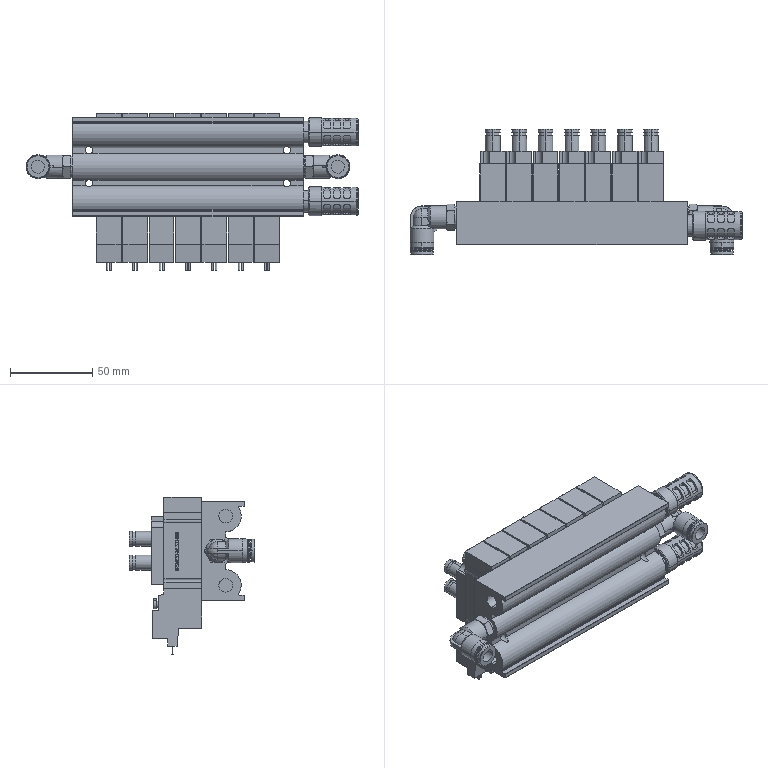Part | NX | 12 solids | 4892 faces | volume 410656 mm3 | plane 4170 | cylinder 576 | cone 132 | torus 8 | sphere 4 | spline 2 | commonest cylinder face diameters 2 x96 4 x84 9 x56 2.5 x42 7.938 x42 14 x36